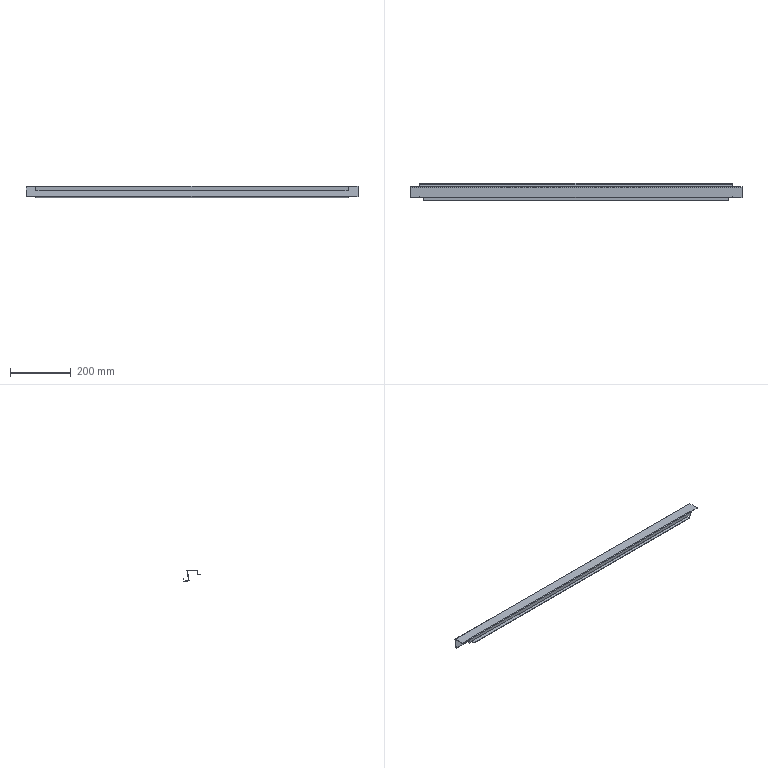Part | SolidWorks | features EdgeFlange 5, FlatPattern 1, SMBaseFlange 1, SheetMetal 1 | 1 solid | 70 faces | box 1097 x 57.715 x 37.08 mm | volume 185139 mm3 | plane 60 | cylinder 10 | commonest cylinder face diameters 0.2 x5 3.2 x5